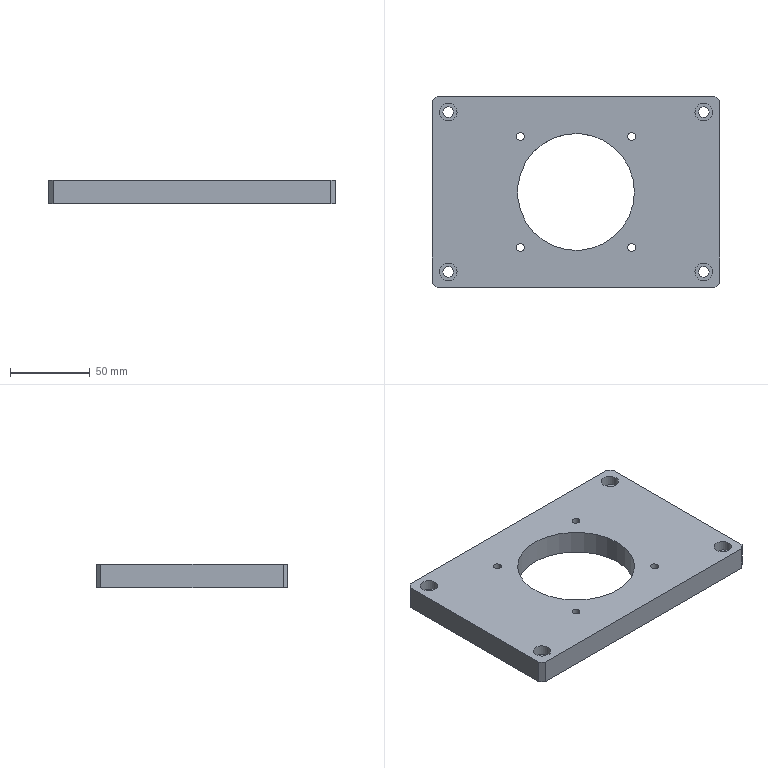CAM job | NX | 3-axis milling, drilling | part box 180 x 120 x 15 mm | stock box 185 x 125 x 20 mm
Tools:
number,name,description,diameter,corner_radius,flute_length,length,flutes
6,D6,平底铣刀-粗,6.0,0.0,25.0,75.0,2
9,D10,平底铣刀-粗,10.0,0.0,35.0,75.0,2
7,D6-J,平底铣刀-精,6.0,0.0,25.0,75.0,2
10,D10-J,平底铣刀-精,10.0,0.0,35.0,75.0,2
1,D80R0.8飞刀,圆鼻刀-粗,80.0,0.8,50.0,75.0,2
1,D80R0.8飞刀-J,圆鼻刀-精,80.0,0.8,50.0,75.0,2
2,D6倒角刀,倒角刀,6.0,0.0,3.0,25.0,2
19,M6X1.0,丝锥,5.0,0.0,35.0,50.0,2
15,ZT5,钻头,5.0,0.0,35.0,50.0,2
17,ZT6.6,钻头,6.6,0.0,35.0,50.0,2
Operations:
program,operation,operation_type,tool,method,geometry_group,spindle_rpm,surface_speed,feed_per_tooth,feed_cut,feed_plunge,cut_length_mm,path_length_mm,cut_time_min,machine_time_min
B,底壁铣飞面开粗_COPY,VolumeBased25DMillingOperation,D80R0.8飞刀,分层开粗-切深K-步距G,W-B,2800.0,703.696,0.5357,3000.0,100.0,5457.187,6007.757,1.819,1.874
B,底壁铣飞面精光_COPY,VolumeBased25DMillingOperation,D80R0.8飞刀-J,侧刃精光-切深K-步距G,W-B,4000.0,1005.28,0.125,1000.0,100.0,859.584,895.584,0.8596,0.8632
B,铣倒角_4,PlanarMilling,D6倒角刀,METHOD,W-B,8000.0,150.796,0.0375,600.0,100.0,75.821,451.843,0.1264,0.164
B,铣倒角_5,PlanarMilling,D6倒角刀,METHOD,W-B,8000.0,150.796,0.075,1200.0,100.0,81.784,608.999,0.0682,0.1209
B,C0.3封闭铣廓倒角6X45L_COPY,PlanarMilling,D6倒角刀,爬面_倒角-切深0-步距G,W-B,7000.0,131.0,0.1071,1500.0,100.0,849.298,1008.936,0.5662,0.5822
A,顶面,FaceMilling,D80R0.8飞刀,侧刃精光-切深K-步距G,W-A,4000.0,1005.31,0.125,1000.0,100.0,894.0,930.0,0.894,0.8976
A,外形粗_2,VolumeBased25DMillingOperation,D10,METHOD,W-A,8000.0,251.327,0.3125,5000.0,80.0,13126.821,13180.821,2.625,2.631
A,底壁铣螺旋开粗-中_COPY,VolumeBased25DMillingOperation,D10,分层开粗-切深K-步距G,W-A,8000.0,251.32,0.25,4000.0,100.0,5166.458,5219.258,1.292,1.297
A,打点-深0.8,Operation,D6倒角刀,NONE,W-A,8000.0,150.796,0.0312,500.0,90.0,14.4,505.811,0.0288,0.0779
A,通孔-M6螺纹底孔,Operation,ZT5,NONE,W-A,2800.0,43.982,0.0625,350.0,90.0,94.009,439.839,0.2686,0.3032
A,沉头孔-钻孔0段,Operation,ZT6.6,NONE,W-A,1200.0,24.881,0.0625,150.0,90.0,79.931,562.876,0.5329,0.5812
A,铣孔开粗D6_1,CylinderMilling,D6,NONE,W-A,8000.0,150.796,0.075,1200.0,100.0,923.332,1466.932,0.7694,0.8238
A,铣孔精光D6_1,CylinderMilling,D6-J,精光步距切深关,W-A,8000.0,150.796,0.0312,500.0,100.0,178.461,724.061,0.3569,0.4115
A,仅选体,SurfaceContour,D6倒角刀,METHOD,W-A,8000.0,150.796,0.1875,3000.0,100.0,841.247,983.758,0.2804,0.2947
A,铣倒角_1,PlanarMilling,D6倒角刀,METHOD,W-A,8000.0,150.796,0.0312,500.0,100.0,73.926,446.744,0.1479,0.1851
A,铣倒角_2,PlanarMilling,D6倒角刀,NONE,W-A,8000.0,150.796,0.05,800.0,100.0,173.57,684.885,0.217,0.2681
A,铣倒角_3,PlanarMilling,D6倒角刀,METHOD,W-A,8000.0,150.796,0.0312,500.0,100.0,79.753,451.37,0.1595,0.1967
A,通孔-攻牙M6,Operation,M6X1.0,METHOD,W-A,500.0,7.854,0.001,1.0,90.0,78.0,407.822,78.0,78.033
A,底壁铣精光侧面-中_COPY,VolumeBased25DMillingOperation,D6-J,侧刃精光-切深K-步距G,W-A,6000.0,113.097,0.0833,1000.0,100.0,435.534,483.451,0.4355,0.4403
A,外形半精_2,VolumeBased25DMillingOperation,D10-J,METHOD,W-A,8000.0,251.327,0.0625,1000.0,100.0,629.31,699.31,0.6293,0.6363